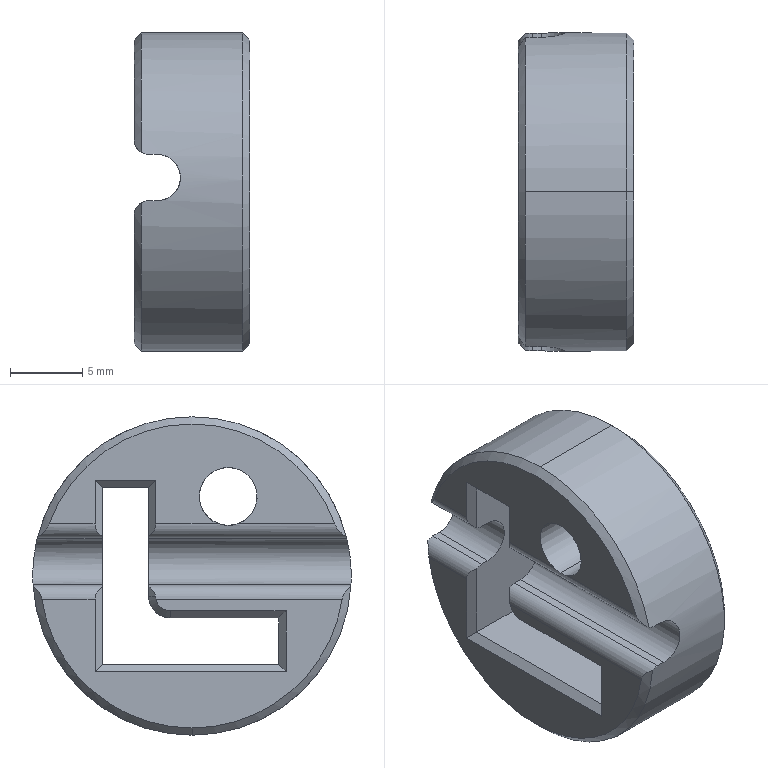Part | SolidWorks | features BaseBody 1 | 1 solid | 45 faces | box 8 x 22 x 22 mm | volume 2188 mm3 | plane 27 | cylinder 11 | cone 7 | commonest cylinder face diameters 2 x4 3.2 x2 4 x2 22 x2 3 x1
STEP:
#1=CARTESIAN_POINT('',(16.,98.,-26.5));
#2=VERTEX_POINT('',#1);
#3=CARTESIAN_POINT('',(16.,98.,-5.5));
#4=VERTEX_POINT('',#3);
#5=CARTESIAN_POINT('',(16.,98.,-16.));
#6=DIRECTION('',(1.,0.,0.));
#7=DIRECTION('',(0.,0.,1.));
#8=AXIS2_PLACEMENT_3D('',#5,#6,#7);
#9=CIRCLE('',#8,10.5);
#10=EDGE_CURVE('',#2,#4,#9,.T.);
#11=ORIENTED_EDGE('',*,*,#10,.F.);
#12=CARTESIAN_POINT('',(15.5,98.,-27.));
#13=VERTEX_POINT('',#12);
#14=CARTESIAN_POINT('',(15.5,98.,-27.));
#15=DIRECTION('',(-0.7071,0.,-0.7071));
#16=VECTOR('',#15,1000.);
#17=LINE('',#14,#16);
#18=EDGE_CURVE('',#2,#13,#17,.T.);
#19=ORIENTED_EDGE('',*,*,#18,.T.);
#20=CARTESIAN_POINT('',(15.5,98.,-5.));
#21=VERTEX_POINT('',#20);
#22=CARTESIAN_POINT('',(15.5,98.,-16.));
#23=DIRECTION('',(-1.,0.,0.));
#24=DIRECTION('',(0.,0.,1.));
#25=AXIS2_PLACEMENT_3D('',#22,#23,#24);
#26=CIRCLE('',#25,11.);
#27=EDGE_CURVE('',#21,#13,#26,.T.);
#28=ORIENTED_EDGE('',*,*,#27,.F.);
#29=CARTESIAN_POINT('',(15.5,98.,-5.));
#30=DIRECTION('',(-0.7071,0.,0.7071));
#31=VECTOR('',#30,1000.);
#32=LINE('',#29,#31);
#33=EDGE_CURVE('',#4,#21,#32,.T.);
#34=ORIENTED_EDGE('',*,*,#33,.F.);
#35=EDGE_LOOP('',(#11,#19,#28,#34));
#36=FACE_OUTER_BOUND('',#35,.T.);
#37=CARTESIAN_POINT('',(15.5,98.,-16.));
#38=DIRECTION('',(-1.,0.,0.));
#39=DIRECTION('',(0.,0.,1.));
#40=AXIS2_PLACEMENT_3D('',#37,#38,#39);
#41=CONICAL_SURFACE('',#40,11.,0.7854);
#42=ADVANCED_FACE('',(#36),#41,.T.);
#43=CARTESIAN_POINT('',(8.,94.876,-12.4));
#44=VERTEX_POINT('',#43);
#45=CARTESIAN_POINT('',(8.,95.5,-8.5));
#46=VERTEX_POINT('',#45);
#47=CARTESIAN_POINT('',(8.,95.5,-10.5));
#48=DIRECTION('',(-1.,0.,0.));
#49=DIRECTION('',(0.,0.,1.));
#50=AXIS2_PLACEMENT_3D('',#47,#48,#49);
#51=CIRCLE('',#50,2.);
#52=EDGE_CURVE('',#44,#46,#51,.T.);
#53=ORIENTED_EDGE('',*,*,#52,.T.);
#54=CARTESIAN_POINT('',(16.,95.5,-8.5));
#55=VERTEX_POINT('',#54);
#56=CARTESIAN_POINT('',(8.,95.5,-8.5));
#57=DIRECTION('',(1.,0.,0.));
#58=VECTOR('',#57,1000.);
#59=LINE('',#56,#58);
#60=EDGE_CURVE('',#46,#55,#59,.T.);
#61=ORIENTED_EDGE('',*,*,#60,.T.);
#62=CARTESIAN_POINT('',(16.,95.5,-12.5));
#63=VERTEX_POINT('',#62);
#64=CARTESIAN_POINT('',(16.,95.5,-10.5));
#65=DIRECTION('',(-1.,0.,0.));
#66=DIRECTION('',(0.,0.,1.));
#67=AXIS2_PLACEMENT_3D('',#64,#65,#66);
#68=CIRCLE('',#67,2.);
#69=EDGE_CURVE('',#63,#55,#68,.T.);
#70=ORIENTED_EDGE('',*,*,#69,.F.);
#71=CARTESIAN_POINT('',(8.005,95.5,-12.5));
#72=VERTEX_POINT('',#71);
#73=CARTESIAN_POINT('',(8.,95.5,-12.5));
#74=DIRECTION('',(1.,0.,0.));
#75=VECTOR('',#74,1000.);
#76=LINE('',#73,#75);
#77=EDGE_CURVE('',#72,#63,#76,.T.);
#78=ORIENTED_EDGE('',*,*,#77,.F.);
#79=CARTESIAN_POINT('',(8.005,95.5,-12.5));
#80=CARTESIAN_POINT('',(8.005,95.287,-12.5));
#81=CARTESIAN_POINT('',(8.,95.078,-12.467));
#82=CARTESIAN_POINT('',(8.,94.876,-12.4));
#83=B_SPLINE_CURVE_WITH_KNOTS('',3,(#79,#80,#81,#82),.UNSPECIFIED.,.F.,.F.,(4,4),(0.0006324,0.001263),.UNSPECIFIED.);
#84=EDGE_CURVE('',#72,#44,#83,.T.);
#85=ORIENTED_EDGE('',*,*,#84,.T.);
#86=EDGE_LOOP('',(#53,#61,#70,#78,#85));
#87=FACE_OUTER_BOUND('',#86,.T.);
#88=CARTESIAN_POINT('',(8.,95.5,-10.5));
#89=DIRECTION('',(1.,0.,0.));
#90=DIRECTION('',(0.,0.,-1.));
#91=AXIS2_PLACEMENT_3D('',#88,#89,#90);
#92=CYLINDRICAL_SURFACE('',#91,2.);
#93=ADVANCED_FACE('',(#87),#92,.F.);
#94=CARTESIAN_POINT('',(8.5,108.655,-13.266));
#95=VERTEX_POINT('',#94);
#96=CARTESIAN_POINT('',(8.5,98.,-5.));
#97=VERTEX_POINT('',#96);
#98=CARTESIAN_POINT('',(8.5,98.,-16.));
#99=DIRECTION('',(1.,0.,0.));
#100=DIRECTION('',(0.,0.,1.));
#101=AXIS2_PLACEMENT_3D('',#98,#99,#100);
#102=CIRCLE('',#101,11.);
#103=EDGE_CURVE('',#95,#97,#102,.T.);
#104=ORIENTED_EDGE('',*,*,#103,.T.);
#105=CARTESIAN_POINT('',(8.,98.,-5.));
#106=DIRECTION('',(1.,0.,0.));
#107=VECTOR('',#106,1000.);
#108=LINE('',#105,#107);
#109=EDGE_CURVE('',#97,#21,#108,.T.);
#110=ORIENTED_EDGE('',*,*,#109,.T.);
#111=ORIENTED_EDGE('',*,*,#27,.T.);
#112=CARTESIAN_POINT('',(8.5,98.,-27.));
#113=VERTEX_POINT('',#112);
#114=CARTESIAN_POINT('',(8.,98.,-27.));
#115=DIRECTION('',(1.,0.,0.));
#116=VECTOR('',#115,1000.);
#117=LINE('',#114,#116);
#118=EDGE_CURVE('',#113,#13,#117,.T.);
#119=ORIENTED_EDGE('',*,*,#118,.F.);
#120=CARTESIAN_POINT('',(8.5,108.975,-16.734));
#121=VERTEX_POINT('',#120);
#122=CARTESIAN_POINT('',(8.5,98.,-16.));
#123=DIRECTION('',(1.,0.,0.));
#124=DIRECTION('',(0.,0.,1.));
#125=AXIS2_PLACEMENT_3D('',#122,#123,#124);
#126=CIRCLE('',#125,11.);
#127=EDGE_CURVE('',#113,#121,#126,.T.);
#128=ORIENTED_EDGE('',*,*,#127,.T.);
#129=CARTESIAN_POINT('',(9.,108.984,-16.6));
#130=VERTEX_POINT('',#129);
#131=CARTESIAN_POINT('',(8.5,108.975,-16.734));
#132=CARTESIAN_POINT('',(8.652,108.981,-16.646));
#133=CARTESIAN_POINT('',(8.824,108.984,-16.6));
#134=CARTESIAN_POINT('',(9.,108.984,-16.6));
#135=B_SPLINE_CURVE_WITH_KNOTS('',3,(#131,#132,#133,#134),.UNSPECIFIED.,.F.,.F.,(4,4),(0.,0.00052),.UNSPECIFIED.);
#136=EDGE_CURVE('',#121,#130,#135,.T.);
#137=ORIENTED_EDGE('',*,*,#136,.T.);
#138=CARTESIAN_POINT('',(9.6,108.984,-16.6));
#139=VERTEX_POINT('',#138);
#140=CARTESIAN_POINT('',(8.,108.984,-16.6));
#141=DIRECTION('',(1.,0.,0.));
#142=VECTOR('',#141,1000.);
#143=LINE('',#140,#142);
#144=EDGE_CURVE('',#130,#139,#143,.T.);
#145=ORIENTED_EDGE('',*,*,#144,.T.);
#146=CARTESIAN_POINT('',(9.6,108.688,-13.4));
#147=VERTEX_POINT('',#146);
#148=CARTESIAN_POINT('',(9.6,108.984,-16.6));
#149=CARTESIAN_POINT('',(9.706,108.984,-16.6));
#150=CARTESIAN_POINT('',(9.81,108.984,-16.59));
#151=CARTESIAN_POINT('',(10.015,108.986,-16.549));
#152=CARTESIAN_POINT('',(10.117,108.988,-16.518));
#153=CARTESIAN_POINT('',(10.312,108.991,-16.437));
#154=CARTESIAN_POINT('',(10.404,108.993,-16.387));
#155=CARTESIAN_POINT('',(10.578,108.997,-16.271));
#156=CARTESIAN_POINT('',(10.661,108.998,-16.203));
#157=CARTESIAN_POINT('',(10.882,109.001,-15.98));
#158=CARTESIAN_POINT('',(11.001,109.,-15.8));
#159=CARTESIAN_POINT('',(11.16,108.986,-15.414));
#160=CARTESIAN_POINT('',(11.201,108.973,-15.202));
#161=CARTESIAN_POINT('',(11.2,108.944,-14.889));
#162=CARTESIAN_POINT('',(11.189,108.933,-14.784));
#163=CARTESIAN_POINT('',(11.147,108.908,-14.58));
#164=CARTESIAN_POINT('',(11.117,108.895,-14.48));
#165=CARTESIAN_POINT('',(10.996,108.852,-14.191));
#166=CARTESIAN_POINT('',(10.88,108.821,-14.017));
#167=CARTESIAN_POINT('',(10.657,108.777,-13.794));
#168=CARTESIAN_POINT('',(10.577,108.763,-13.728));
#169=CARTESIAN_POINT('',(10.404,108.738,-13.613));
#170=CARTESIAN_POINT('',(10.311,108.727,-13.563));
#171=CARTESIAN_POINT('',(10.021,108.699,-13.442));
#172=CARTESIAN_POINT('',(9.812,108.688,-13.4));
#173=CARTESIAN_POINT('',(9.6,108.688,-13.4));
#174=B_SPLINE_CURVE_WITH_KNOTS('',3,(#148,#149,#150,#151,#152,#153,#154,#155,#156,#157,#158,#159,#160,#161,#162,#163,#164,#165,#166,#167,#168,#169,#170,#171,#172,#173),.UNSPECIFIED.,.F.,.F.,(4,2,2,2,2,2,2,2,2,2,2,2,4),(0.,0.0003137,0.0006273,0.000941,0.001255,0.001882,0.002509,0.002823,0.003137,0.003764,0.004078,0.004391,0.005019),.UNSPECIFIED.);
#175=EDGE_CURVE('',#139,#147,#174,.T.);
#176=ORIENTED_EDGE('',*,*,#175,.T.);
#177=CARTESIAN_POINT('',(9.,108.688,-13.4));
#178=VERTEX_POINT('',#177);
#179=CARTESIAN_POINT('',(8.,108.688,-13.4));
#180=DIRECTION('',(-1.,0.,0.));
#181=VECTOR('',#180,1000.);
#182=LINE('',#179,#181);
#183=EDGE_CURVE('',#147,#178,#182,.T.);
#184=ORIENTED_EDGE('',*,*,#183,.T.);
#185=CARTESIAN_POINT('',(9.,108.688,-13.4));
#186=CARTESIAN_POINT('',(8.824,108.688,-13.4));
#187=CARTESIAN_POINT('',(8.651,108.677,-13.353));
#188=CARTESIAN_POINT('',(8.5,108.655,-13.266));
#189=B_SPLINE_CURVE_WITH_KNOTS('',3,(#185,#186,#187,#188),.UNSPECIFIED.,.F.,.F.,(4,4),(0.,0.0005213),.UNSPECIFIED.);
#190=EDGE_CURVE('',#178,#95,#189,.T.);
#191=ORIENTED_EDGE('',*,*,#190,.T.);
#192=EDGE_LOOP('',(#104,#110,#111,#119,#128,#137,#145,#176,#184,#191));
#193=FACE_OUTER_BOUND('',#192,.T.);
#194=CARTESIAN_POINT('',(8.,98.,-16.));
#195=DIRECTION('',(1.,0.,0.));
#196=DIRECTION('',(0.,0.,-1.));
#197=AXIS2_PLACEMENT_3D('',#194,#195,#196);
#198=CYLINDRICAL_SURFACE('',#197,11.);
#199=ADVANCED_FACE('',(#193),#198,.T.);
#200=CARTESIAN_POINT('',(8.,98.,-26.5));
#201=VERTEX_POINT('',#200);
#202=CARTESIAN_POINT('',(8.,87.623,-17.6));
#203=VERTEX_POINT('',#202);
#204=CARTESIAN_POINT('',(8.,98.,-16.));
#205=DIRECTION('',(-1.,0.,0.));
#206=DIRECTION('',(0.,0.,1.));
#207=AXIS2_PLACEMENT_3D('',#204,#205,#206);
#208=CIRCLE('',#207,10.5);
#209=EDGE_CURVE('',#201,#203,#208,.T.);
#210=ORIENTED_EDGE('',*,*,#209,.F.);
#211=CARTESIAN_POINT('',(8.,98.,-26.5));
#212=DIRECTION('',(0.7071,0.,-0.7071));
#213=VECTOR('',#212,1000.);
#214=LINE('',#211,#213);
#215=EDGE_CURVE('',#201,#113,#214,.T.);
#216=ORIENTED_EDGE('',*,*,#215,.T.);
#217=CARTESIAN_POINT('',(8.5,87.025,-16.734));
#218=VERTEX_POINT('',#217);
#219=CARTESIAN_POINT('',(8.5,98.,-16.));
#220=DIRECTION('',(1.,0.,0.));
#221=DIRECTION('',(0.,0.,1.));
#222=AXIS2_PLACEMENT_3D('',#219,#220,#221);
#223=CIRCLE('',#222,11.);
#224=EDGE_CURVE('',#218,#113,#223,.T.);
#225=ORIENTED_EDGE('',*,*,#224,.F.);
#226=CARTESIAN_POINT('',(8.5,87.025,-16.734));
#227=CARTESIAN_POINT('',(8.434,87.093,-16.772));
#228=CARTESIAN_POINT('',(8.372,87.159,-16.818));
#229=CARTESIAN_POINT('',(8.256,87.284,-16.927));
#230=CARTESIAN_POINT('',(8.202,87.344,-16.991));
#231=CARTESIAN_POINT('',(8.063,87.505,-17.21));
#232=CARTESIAN_POINT('',(8.,87.591,-17.396));
#233=CARTESIAN_POINT('',(8.,87.623,-17.6));
#234=B_SPLINE_CURVE_WITH_KNOTS('',3,(#226,#227,#228,#229,#230,#231,#232,#233),.UNSPECIFIED.,.F.,.F.,(4,2,2,4),(0.,0.0003033,0.0006065,0.001213),.UNSPECIFIED.);
#235=EDGE_CURVE('',#218,#203,#234,.T.);
#236=ORIENTED_EDGE('',*,*,#235,.T.);
#237=EDGE_LOOP('',(#210,#216,#225,#236));
#238=FACE_OUTER_BOUND('',#237,.T.);
#239=CARTESIAN_POINT('',(8.,98.,-16.));
#240=DIRECTION('',(1.,0.,0.));
#241=DIRECTION('',(0.,0.,-1.));
#242=AXIS2_PLACEMENT_3D('',#239,#240,#241);
#243=CONICAL_SURFACE('',#242,10.5,0.7854);
#244=ADVANCED_FACE('',(#238),#243,.T.);
#245=CARTESIAN_POINT('',(8.,108.377,-17.6));
#246=VERTEX_POINT('',#245);
#247=CARTESIAN_POINT('',(8.,98.,-16.));
#248=DIRECTION('',(-1.,0.,0.));
#249=DIRECTION('',(0.,0.,1.));
#250=AXIS2_PLACEMENT_3D('',#247,#248,#249);
#251=CIRCLE('',#250,10.5);
#252=EDGE_CURVE('',#246,#201,#251,.T.);
#253=ORIENTED_EDGE('',*,*,#252,.T.);
#254=ORIENTED_EDGE('',*,*,#209,.T.);
#255=CARTESIAN_POINT('',(8.,100.48,-17.6));
#256=VERTEX_POINT('',#255);
#257=CARTESIAN_POINT('',(8.,100.5,-17.6));
#258=DIRECTION('',(0.,1.,0.));
#259=VECTOR('',#258,1000.);
#260=LINE('',#257,#259);
#261=EDGE_CURVE('',#203,#256,#260,.T.);
#262=ORIENTED_EDGE('',*,*,#261,.T.);
#263=CARTESIAN_POINT('',(8.,99.5,-18.4));
#264=VERTEX_POINT('',#263);
#265=CARTESIAN_POINT('',(8.,99.5,-17.4));
#266=DIRECTION('',(-1.,0.,0.));
#267=DIRECTION('',(0.,0.,1.));
#268=AXIS2_PLACEMENT_3D('',#265,#266,#267);
#269=CIRCLE('',#268,1.);
#270=EDGE_CURVE('',#256,#264,#269,.T.);
#271=ORIENTED_EDGE('',*,*,#270,.T.);
#272=CARTESIAN_POINT('',(8.,91.5,-18.4));
#273=VERTEX_POINT('',#272);
#274=CARTESIAN_POINT('',(8.,98.,-18.4));
#275=DIRECTION('',(0.,-1.,0.));
#276=VECTOR('',#275,1000.);
#277=LINE('',#274,#276);
#278=EDGE_CURVE('',#264,#273,#277,.T.);
#279=ORIENTED_EDGE('',*,*,#278,.T.);
#280=CARTESIAN_POINT('',(8.,91.5,-22.6));
#281=VERTEX_POINT('',#280);
#282=CARTESIAN_POINT('',(8.,91.5,-16.));
#283=DIRECTION('',(0.,0.,-1.));
#284=VECTOR('',#283,1000.);
#285=LINE('',#282,#284);
#286=EDGE_CURVE('',#273,#281,#285,.T.);
#287=ORIENTED_EDGE('',*,*,#286,.T.);
#288=CARTESIAN_POINT('',(8.,104.7,-22.6));
#289=VERTEX_POINT('',#288);
#290=CARTESIAN_POINT('',(8.,98.,-22.6));
#291=DIRECTION('',(0.,1.,0.));
#292=VECTOR('',#291,1000.);
#293=LINE('',#290,#292);
#294=EDGE_CURVE('',#281,#289,#293,.T.);
#295=ORIENTED_EDGE('',*,*,#294,.T.);
#296=CARTESIAN_POINT('',(8.,104.7,-17.6));
#297=VERTEX_POINT('',#296);
#298=CARTESIAN_POINT('',(8.,104.7,-16.));
#299=DIRECTION('',(0.,0.,1.));
#300=VECTOR('',#299,1000.);
#301=LINE('',#298,#300);
#302=EDGE_CURVE('',#289,#297,#301,.T.);
#303=ORIENTED_EDGE('',*,*,#302,.T.);
#304=CARTESIAN_POINT('',(8.,108.483,-17.6));
#305=DIRECTION('',(0.,1.,0.));
#306=VECTOR('',#305,1000.);
#307=LINE('',#304,#306);
#308=EDGE_CURVE('',#297,#246,#307,.T.);
#309=ORIENTED_EDGE('',*,*,#308,.T.);
#310=EDGE_LOOP('',(#253,#254,#262,#271,#279,#287,#295,#303,#309));
#311=FACE_OUTER_BOUND('',#310,.T.);
#312=CARTESIAN_POINT('',(8.,98.,-16.));
#313=DIRECTION('',(-1.,0.,0.));
#314=DIRECTION('',(0.,0.,1.));
#315=AXIS2_PLACEMENT_3D('',#312,#313,#314);
#316=PLANE('',#315);
#317=ADVANCED_FACE('',(#311),#316,.T.);
#318=ORIENTED_EDGE('',*,*,#215,.F.);
#319=ORIENTED_EDGE('',*,*,#252,.F.);
#320=CARTESIAN_POINT('',(8.,108.377,-17.6));
#321=CARTESIAN_POINT('',(8.,108.409,-17.396));
#322=CARTESIAN_POINT('',(8.062,108.493,-17.212));
#323=CARTESIAN_POINT('',(8.248,108.71,-16.918));
#324=CARTESIAN_POINT('',(8.368,108.838,-16.81));
#325=CARTESIAN_POINT('',(8.5,108.975,-16.734));
#326=B_SPLINE_CURVE_WITH_KNOTS('',3,(#320,#321,#322,#323,#324,#325),.UNSPECIFIED.,.F.,.F.,(4,2,4),(0.,0.0006077,0.001215),.UNSPECIFIED.);
#327=EDGE_CURVE('',#246,#121,#326,.T.);
#328=ORIENTED_EDGE('',*,*,#327,.T.);
#329=ORIENTED_EDGE('',*,*,#127,.F.);
#330=EDGE_LOOP('',(#318,#319,#328,#329));
#331=FACE_OUTER_BOUND('',#330,.T.);
#332=CARTESIAN_POINT('',(8.,98.,-16.));
#333=DIRECTION('',(1.,0.,0.));
#334=DIRECTION('',(0.,0.,-1.));
#335=AXIS2_PLACEMENT_3D('',#332,#333,#334);
#336=CONICAL_SURFACE('',#335,10.5,0.7854);
#337=ADVANCED_FACE('',(#331),#336,.T.);
#338=CARTESIAN_POINT('',(8.02,100.52,-17.4));
#339=VERTEX_POINT('',#338);
#340=CARTESIAN_POINT('',(8.5,101.,-17.4));
#341=VERTEX_POINT('',#340);
#342=CARTESIAN_POINT('',(8.,100.5,-17.4));
#343=DIRECTION('',(0.7071,0.7071,0.));
#344=VECTOR('',#343,1000.);
#345=LINE('',#342,#344);
#346=EDGE_CURVE('',#339,#341,#345,.T.);
#347=ORIENTED_EDGE('',*,*,#346,.F.);
#348=CARTESIAN_POINT('',(8.5,101.,-16.734));
#349=VERTEX_POINT('',#348);
#350=CARTESIAN_POINT('',(8.02,100.52,-17.4));
#351=CARTESIAN_POINT('',(8.078,100.578,-17.115));
#352=CARTESIAN_POINT('',(8.248,100.748,-16.879));
#353=CARTESIAN_POINT('',(8.5,101.,-16.734));
#354=(BOUNDED_CURVE()B_SPLINE_CURVE(3,(#350,#351,#352,#353),.UNSPECIFIED.,.F.,.F.)B_SPLINE_CURVE_WITH_KNOTS((4,4),(0.2014,1.047),.UNSPECIFIED.)CURVE()GEOMETRIC_REPRESENTATION_ITEM()RATIONAL_B_SPLINE_CURVE((1.,0.9413,0.9413,1.))REPRESENTATION_ITEM(''));
#355=EDGE_CURVE('',#339,#349,#354,.T.);
#356=ORIENTED_EDGE('',*,*,#355,.T.);
#357=CARTESIAN_POINT('',(8.5,101.,-17.4));
#358=DIRECTION('',(0.,0.,1.));
#359=VECTOR('',#358,1000.);
#360=LINE('',#357,#359);
#361=EDGE_CURVE('',#341,#349,#360,.T.);
#362=ORIENTED_EDGE('',*,*,#361,.F.);
#363=EDGE_LOOP('',(#347,#356,#362));
#364=FACE_OUTER_BOUND('',#363,.T.);
#365=CARTESIAN_POINT('',(8.5,101.,-17.4));
#366=DIRECTION('',(0.7071,-0.7071,0.));
#367=DIRECTION('',(0.7071,0.7071,0.));
#368=AXIS2_PLACEMENT_3D('',#365,#366,#367);
#369=PLANE('',#368);
#370=ADVANCED_FACE('',(#364),#369,.F.);
#371=CARTESIAN_POINT('',(8.5,104.2,-16.734));
#372=VERTEX_POINT('',#371);
#373=CARTESIAN_POINT('',(8.5,104.2,-22.1));
#374=VERTEX_POINT('',#373);
#375=CARTESIAN_POINT('',(8.5,104.2,-22.1));
#376=DIRECTION('',(0.,0.,-1.));
#377=VECTOR('',#376,1000.);
#378=LINE('',#375,#377);
#379=EDGE_CURVE('',#372,#374,#378,.T.);
#380=ORIENTED_EDGE('',*,*,#379,.F.);
#381=CARTESIAN_POINT('',(8.5,104.2,-16.734));
#382=CARTESIAN_POINT('',(8.183,104.517,-16.917));
#383=CARTESIAN_POINT('',(8.,104.7,-17.234));
#384=CARTESIAN_POINT('',(8.,104.7,-17.6));
#385=(BOUNDED_CURVE()B_SPLINE_CURVE(3,(#381,#382,#383,#384),.UNSPECIFIED.,.F.,.F.)B_SPLINE_CURVE_WITH_KNOTS((4,4),(2.094,3.142),.UNSPECIFIED.)CURVE()GEOMETRIC_REPRESENTATION_ITEM()RATIONAL_B_SPLINE_CURVE((1.,0.9107,0.9107,1.))REPRESENTATION_ITEM(''));
#386=EDGE_CURVE('',#372,#297,#385,.T.);
#387=ORIENTED_EDGE('',*,*,#386,.T.);
#388=ORIENTED_EDGE('',*,*,#302,.F.);
#389=CARTESIAN_POINT('',(8.5,104.2,-22.1));
#390=DIRECTION('',(-0.5774,0.5774,-0.5774));
#391=VECTOR('',#390,1000.);
#392=LINE('',#389,#391);
#393=EDGE_CURVE('',#374,#289,#392,.T.);
#394=ORIENTED_EDGE('',*,*,#393,.F.);
#395=EDGE_LOOP('',(#380,#387,#388,#394));
#396=FACE_OUTER_BOUND('',#395,.T.);
#397=CARTESIAN_POINT('',(8.5,104.2,-22.1));
#398=DIRECTION('',(0.7071,0.7071,0.));
#399=DIRECTION('',(-0.7071,0.7071,0.));
#400=AXIS2_PLACEMENT_3D('',#397,#398,#399);
#401=PLANE('',#400);
#402=ADVANCED_FACE('',(#396),#401,.F.);
#403=CARTESIAN_POINT('',(8.,88.136,-12.4));
#404=VERTEX_POINT('',#403);
#405=CARTESIAN_POINT('',(8.,107.864,-12.4));
#406=VERTEX_POINT('',#405);
#407=CARTESIAN_POINT('',(8.,98.,-16.));
#408=DIRECTION('',(-1.,0.,0.));
#409=DIRECTION('',(0.,0.,1.));
#410=AXIS2_PLACEMENT_3D('',#407,#408,#409);
#411=CIRCLE('',#410,10.5);
#412=EDGE_CURVE('',#404,#406,#411,.T.);
#413=ORIENTED_EDGE('',*,*,#412,.T.);
#414=CARTESIAN_POINT('',(8.,104.7,-12.4));
#415=VERTEX_POINT('',#414);
#416=CARTESIAN_POINT('',(8.,104.7,-12.4));
#417=DIRECTION('',(0.,-1.,0.));
#418=VECTOR('',#417,1000.);
#419=LINE('',#416,#418);
#420=EDGE_CURVE('',#406,#415,#419,.T.);
#421=ORIENTED_EDGE('',*,*,#420,.T.);
#422=CARTESIAN_POINT('',(8.,104.7,-9.4));
#423=VERTEX_POINT('',#422);
#424=CARTESIAN_POINT('',(8.,104.7,-16.));
#425=DIRECTION('',(0.,0.,1.));
#426=VECTOR('',#425,1000.);
#427=LINE('',#424,#426);
#428=EDGE_CURVE('',#415,#423,#427,.T.);
#429=ORIENTED_EDGE('',*,*,#428,.T.);
#430=CARTESIAN_POINT('',(8.,100.5,-9.4));
#431=VERTEX_POINT('',#430);
#432=CARTESIAN_POINT('',(8.,98.,-9.4));
#433=DIRECTION('',(0.,-1.,0.));
#434=VECTOR('',#433,1000.);
#435=LINE('',#432,#434);
#436=EDGE_CURVE('',#423,#431,#435,.T.);
#437=ORIENTED_EDGE('',*,*,#436,.T.);
#438=CARTESIAN_POINT('',(8.,100.5,-12.4));
#439=VERTEX_POINT('',#438);
#440=CARTESIAN_POINT('',(8.,100.5,-16.));
#441=DIRECTION('',(0.,0.,-1.));
#442=VECTOR('',#441,1000.);
#443=LINE('',#440,#442);
#444=EDGE_CURVE('',#431,#439,#443,.T.);
#445=ORIENTED_EDGE('',*,*,#444,.T.);
#446=CARTESIAN_POINT('',(8.,96.124,-12.4));
#447=VERTEX_POINT('',#446);
#448=CARTESIAN_POINT('',(8.,87.827,-12.4));
#449=DIRECTION('',(0.,-1.,0.));
#450=VECTOR('',#449,1000.);
#451=LINE('',#448,#450);
#452=EDGE_CURVE('',#439,#447,#451,.T.);
#453=ORIENTED_EDGE('',*,*,#452,.T.);
#454=CARTESIAN_POINT('',(8.,95.5,-10.5));
#455=DIRECTION('',(-1.,0.,0.));
#456=DIRECTION('',(0.,0.,1.));
#457=AXIS2_PLACEMENT_3D('',#454,#455,#456);
#458=CIRCLE('',#457,2.);
#459=EDGE_CURVE('',#46,#447,#458,.T.);
#460=ORIENTED_EDGE('',*,*,#459,.F.);
#461=ORIENTED_EDGE('',*,*,#52,.F.);
#462=CARTESIAN_POINT('',(8.,87.827,-12.4));
#463=DIRECTION('',(0.,-1.,0.));
#464=VECTOR('',#463,1000.);
#465=LINE('',#462,#464);
#466=EDGE_CURVE('',#44,#404,#465,.T.);
#467=ORIENTED_EDGE('',*,*,#466,.T.);
#468=EDGE_LOOP('',(#413,#421,#429,#437,#445,#453,#460,#461,#467));
#469=FACE_OUTER_BOUND('',#468,.T.);
#470=CARTESIAN_POINT('',(8.,98.,-16.));
#471=DIRECTION('',(-1.,0.,0.));
#472=DIRECTION('',(0.,0.,1.));
#473=AXIS2_PLACEMENT_3D('',#470,#471,#472);
#474=PLANE('',#473);
#475=ADVANCED_FACE('',(#469),#474,.T.);
#476=CARTESIAN_POINT('',(16.,98.,-16.));
#477=DIRECTION('',(1.,0.,0.));
#478=DIRECTION('',(0.,0.,1.));
#479=AXIS2_PLACEMENT_3D('',#476,#477,#478);
#480=CIRCLE('',#479,10.5);
#481=EDGE_CURVE('',#4,#2,#480,.T.);
#482=ORIENTED_EDGE('',*,*,#481,.T.);
#483=ORIENTED_EDGE('',*,*,#10,.T.);
#484=EDGE_LOOP('',(#482,#483));
#485=FACE_OUTER_BOUND('',#484,.T.);
#486=CARTESIAN_POINT('',(16.,100.5,-9.4));
#487=VERTEX_POINT('',#486);
#488=CARTESIAN_POINT('',(16.,104.7,-9.4));
#489=VERTEX_POINT('',#488);
#490=CARTESIAN_POINT('',(16.,104.2,-9.4));
#491=DIRECTION('',(0.,1.,0.));
#492=VECTOR('',#491,1000.);
#493=LINE('',#490,#492);
#494=EDGE_CURVE('',#487,#489,#493,.T.);
#495=ORIENTED_EDGE('',*,*,#494,.T.);
#496=CARTESIAN_POINT('',(16.,104.7,-22.6));
#497=VERTEX_POINT('',#496);
#498=CARTESIAN_POINT('',(16.,104.7,-22.1));
#499=DIRECTION('',(0.,0.,-1.));
#500=VECTOR('',#499,1000.);
#501=LINE('',#498,#500);
#502=EDGE_CURVE('',#489,#497,#501,.T.);
#503=ORIENTED_EDGE('',*,*,#502,.T.);
#504=CARTESIAN_POINT('',(16.,91.5,-22.6));
#505=VERTEX_POINT('',#504);
#506=CARTESIAN_POINT('',(16.,92.,-22.6));
#507=DIRECTION('',(0.,-1.,0.));
#508=VECTOR('',#507,1000.);
#509=LINE('',#506,#508);
#510=EDGE_CURVE('',#497,#505,#509,.T.);
#511=ORIENTED_EDGE('',*,*,#510,.T.);
#512=CARTESIAN_POINT('',(16.,91.5,-18.4));
#513=VERTEX_POINT('',#512);
#514=CARTESIAN_POINT('',(16.,91.5,-18.9));
#515=DIRECTION('',(0.,0.,1.));
#516=VECTOR('',#515,1000.);
#517=LINE('',#514,#516);
#518=EDGE_CURVE('',#505,#513,#517,.T.);
#519=ORIENTED_EDGE('',*,*,#518,.T.);
#520=CARTESIAN_POINT('',(16.,99.5,-18.4));
#521=VERTEX_POINT('',#520);
#522=CARTESIAN_POINT('',(16.,99.5,-18.4));
#523=DIRECTION('',(0.,1.,0.));
#524=VECTOR('',#523,1000.);
#525=LINE('',#522,#524);
#526=EDGE_CURVE('',#513,#521,#525,.T.);
#527=ORIENTED_EDGE('',*,*,#526,.T.);
#528=CARTESIAN_POINT('',(16.,100.5,-17.4));
#529=VERTEX_POINT('',#528);
#530=CARTESIAN_POINT('',(16.,99.5,-17.4));
#531=DIRECTION('',(1.,0.,0.));
#532=DIRECTION('',(0.,0.,1.));
#533=AXIS2_PLACEMENT_3D('',#530,#531,#532);
#534=CIRCLE('',#533,1.);
#535=EDGE_CURVE('',#521,#529,#534,.T.);
#536=ORIENTED_EDGE('',*,*,#535,.T.);
#537=CARTESIAN_POINT('',(16.,100.5,-9.9));
#538=DIRECTION('',(0.,0.,1.));
#539=VECTOR('',#538,1000.);
#540=LINE('',#537,#539);
#541=EDGE_CURVE('',#529,#487,#540,.T.);
#542=ORIENTED_EDGE('',*,*,#541,.T.);
#543=EDGE_LOOP('',(#495,#503,#511,#519,#527,#536,#542));
#544=FACE_BOUND('',#543,.T.);
#545=ORIENTED_EDGE('',*,*,#69,.T.);
#546=CARTESIAN_POINT('',(16.,95.5,-10.5));
#547=DIRECTION('',(-1.,0.,0.));
#548=DIRECTION('',(0.,0.,1.));
#549=AXIS2_PLACEMENT_3D('',#546,#547,#548);
#550=CIRCLE('',#549,2.);
#551=EDGE_CURVE('',#55,#63,#550,.T.);
#552=ORIENTED_EDGE('',*,*,#551,.T.);
#553=EDGE_LOOP('',(#545,#552));
#554=FACE_BOUND('',#553,.T.);
#555=CARTESIAN_POINT('',(16.,98.,-16.));
#556=DIRECTION('',(-1.,0.,0.));
#557=DIRECTION('',(0.,0.,1.));
#558=AXIS2_PLACEMENT_3D('',#555,#556,#557);
#559=PLANE('',#558);
#560=ADVANCED_FACE('',(#485,#544,#554),#559,.F.);
#561=ORIENTED_EDGE('',*,*,#109,.F.);
#562=CARTESIAN_POINT('',(8.5,87.345,-13.266));
#563=VERTEX_POINT('',#562);
#564=CARTESIAN_POINT('',(8.5,98.,-16.));
#565=DIRECTION('',(1.,0.,0.));
#566=DIRECTION('',(0.,0.,1.));
#567=AXIS2_PLACEMENT_3D('',#564,#565,#566);
#568=CIRCLE('',#567,11.);
#569=EDGE_CURVE('',#97,#563,#568,.T.);
#570=ORIENTED_EDGE('',*,*,#569,.T.);
#571=CARTESIAN_POINT('',(9.,87.312,-13.4));
#572=VERTEX_POINT('',#571);
#573=CARTESIAN_POINT('',(8.5,87.345,-13.266));
#574=CARTESIAN_POINT('',(8.651,87.323,-13.353));
#575=CARTESIAN_POINT('',(8.824,87.312,-13.4));
#576=CARTESIAN_POINT('',(9.,87.312,-13.4));
#577=B_SPLINE_CURVE_WITH_KNOTS('',3,(#573,#574,#575,#576),.UNSPECIFIED.,.F.,.F.,(4,4),(0.,0.0005213),.UNSPECIFIED.);
#578=EDGE_CURVE('',#563,#572,#577,.T.);
#579=ORIENTED_EDGE('',*,*,#578,.T.);
#580=CARTESIAN_POINT('',(9.6,87.312,-13.4));
#581=VERTEX_POINT('',#580);
#582=CARTESIAN_POINT('',(8.,87.312,-13.4));
#583=DIRECTION('',(1.,0.,0.));
#584=VECTOR('',#583,1000.);
#585=LINE('',#582,#584);
#586=EDGE_CURVE('',#572,#581,#585,.T.);
#587=ORIENTED_EDGE('',*,*,#586,.T.);
#588=CARTESIAN_POINT('',(9.6,87.016,-16.6));
#589=VERTEX_POINT('',#588);
#590=CARTESIAN_POINT('',(9.6,87.312,-13.4));
#591=CARTESIAN_POINT('',(9.706,87.312,-13.4));
#592=CARTESIAN_POINT('',(9.81,87.309,-13.41));
#593=CARTESIAN_POINT('',(10.015,87.299,-13.451));
#594=CARTESIAN_POINT('',(10.117,87.292,-13.482));
#595=CARTESIAN_POINT('',(10.311,87.273,-13.563));
#596=CARTESIAN_POINT('',(10.402,87.262,-13.612));
#597=CARTESIAN_POINT('',(10.576,87.237,-13.728));
#598=CARTESIAN_POINT('',(10.657,87.223,-13.795));
#599=CARTESIAN_POINT('',(10.877,87.18,-14.015));
#600=CARTESIAN_POINT('',(10.996,87.148,-14.192));
#601=CARTESIAN_POINT('',(11.156,87.091,-14.574));
#602=CARTESIAN_POINT('',(11.199,87.066,-14.783));
#603=CARTESIAN_POINT('',(11.201,87.037,-15.096));
#604=CARTESIAN_POINT('',(11.191,87.029,-15.202));
#605=CARTESIAN_POINT('',(11.151,87.015,-15.408));
#606=CARTESIAN_POINT('',(11.121,87.011,-15.508));
#607=CARTESIAN_POINT('',(11.041,87.004,-15.702));
#608=CARTESIAN_POINT('',(10.992,87.002,-15.796));
#609=CARTESIAN_POINT('',(10.876,87.,-15.971));
#610=CARTESIAN_POINT('',(10.81,87.,-16.052));
#611=CARTESIAN_POINT('',(10.661,87.002,-16.203));
#612=CARTESIAN_POINT('',(10.58,87.003,-16.269));
#613=CARTESIAN_POINT('',(10.406,87.007,-16.386));
#614=CARTESIAN_POINT('',(10.312,87.009,-16.437));
#615=CARTESIAN_POINT('',(10.021,87.014,-16.558));
#616=CARTESIAN_POINT('',(9.812,87.016,-16.6));
#617=CARTESIAN_POINT('',(9.6,87.016,-16.6));
#618=B_SPLINE_CURVE_WITH_KNOTS('',3,(#590,#591,#592,#593,#594,#595,#596,#597,#598,#599,#600,#601,#602,#603,#604,#605,#606,#607,#608,#609,#610,#611,#612,#613,#614,#615,#616,#617),.UNSPECIFIED.,.F.,.F.,(4,2,2,2,2,2,2,2,2,2,2,2,2,4),(0.,0.0003137,0.0006273,0.000941,0.001255,0.001882,0.002509,0.002823,0.003137,0.00345,0.003764,0.004078,0.004391,0.005019),.UNSPECIFIED.);
#619=EDGE_CURVE('',#581,#589,#618,.T.);
#620=ORIENTED_EDGE('',*,*,#619,.T.);
#621=CARTESIAN_POINT('',(9.,87.016,-16.6));
#622=VERTEX_POINT('',#621);
#623=CARTESIAN_POINT('',(8.,87.016,-16.6));
#624=DIRECTION('',(-1.,0.,0.));
#625=VECTOR('',#624,1000.);
#626=LINE('',#623,#625);
#627=EDGE_CURVE('',#589,#622,#626,.T.);
#628=ORIENTED_EDGE('',*,*,#627,.T.);
#629=CARTESIAN_POINT('',(9.,87.016,-16.6));
#630=CARTESIAN_POINT('',(8.824,87.016,-16.6));
#631=CARTESIAN_POINT('',(8.652,87.019,-16.646));
#632=CARTESIAN_POINT('',(8.5,87.025,-16.734));
#633=B_SPLINE_CURVE_WITH_KNOTS('',3,(#629,#630,#631,#632),.UNSPECIFIED.,.F.,.F.,(4,4),(0.,0.00052),.UNSPECIFIED.);
#634=EDGE_CURVE('',#622,#218,#633,.T.);
#635=ORIENTED_EDGE('',*,*,#634,.T.);
#636=ORIENTED_EDGE('',*,*,#224,.T.);
#637=ORIENTED_EDGE('',*,*,#118,.T.);
#638=CARTESIAN_POINT('',(15.5,98.,-16.));
#639=DIRECTION('',(-1.,0.,0.));
#640=DIRECTION('',(0.,0.,1.));
#641=AXIS2_PLACEMENT_3D('',#638,#639,#640);
#642=CIRCLE('',#641,11.);
#643=EDGE_CURVE('',#13,#21,#642,.T.);
#644=ORIENTED_EDGE('',*,*,#643,.T.);
#645=EDGE_LOOP('',(#561,#570,#579,#587,#620,#628,#635,#636,#637,#644));
#646=FACE_OUTER_BOUND('',#645,.T.);
#647=CARTESIAN_POINT('',(8.,98.,-16.));
#648=DIRECTION('',(1.,0.,0.));
#649=DIRECTION('',(0.,0.,-1.));
#650=AXIS2_PLACEMENT_3D('',#647,#648,#649);
#651=CYLINDRICAL_SURFACE('',#650,11.);
#652=ADVANCED_FACE('',(#646),#651,.T.);
#653=CARTESIAN_POINT('',(8.5,99.5,-18.9));
#654=VERTEX_POINT('',#653);
#655=CARTESIAN_POINT('',(15.5,99.5,-18.9));
#656=VERTEX_POINT('',#655);
#657=CARTESIAN_POINT('',(8.,99.5,-18.9));
#658=DIRECTION('',(1.,0.,0.));
#659=VECTOR('',#658,1000.);
#660=LINE('',#657,#659);
#661=EDGE_CURVE('',#654,#656,#660,.T.);
#662=ORIENTED_EDGE('',*,*,#661,.F.);
#663=CARTESIAN_POINT('',(8.5,99.5,-17.4));
#664=DIRECTION('',(1.,0.,0.));
#665=DIRECTION('',(0.,0.,1.));
#666=AXIS2_PLACEMENT_3D('',#663,#664,#665);
#667=CIRCLE('',#666,1.5);
#668=EDGE_CURVE('',#654,#341,#667,.T.);
#669=ORIENTED_EDGE('',*,*,#668,.T.);
#670=CARTESIAN_POINT('',(15.5,101.,-17.4));
#671=VERTEX_POINT('',#670);
#672=CARTESIAN_POINT('',(8.,101.,-17.4));
#673=DIRECTION('',(1.,0.,0.));
#674=VECTOR('',#673,1000.);
#675=LINE('',#672,#674);
#676=EDGE_CURVE('',#341,#671,#675,.T.);
#677=ORIENTED_EDGE('',*,*,#676,.T.);
#678=CARTESIAN_POINT('',(15.5,99.5,-17.4));
#679=DIRECTION('',(-1.,0.,0.));
#680=DIRECTION('',(0.,0.,1.));
#681=AXIS2_PLACEMENT_3D('',#678,#679,#680);
#682=CIRCLE('',#681,1.5);
#683=EDGE_CURVE('',#671,#656,#682,.T.);
#684=ORIENTED_EDGE('',*,*,#683,.T.);
#685=EDGE_LOOP('',(#662,#669,#677,#684));
#686=FACE_OUTER_BOUND('',#685,.T.);
#687=CARTESIAN_POINT('',(8.,99.5,-17.4));
#688=DIRECTION('',(1.,0.,0.));
#689=DIRECTION('',(0.,0.,-1.));
#690=AXIS2_PLACEMENT_3D('',#687,#688,#689);
#691=CYLINDRICAL_SURFACE('',#690,1.5);
#692=ADVANCED_FACE('',(#686),#691,.T.);
#693=CARTESIAN_POINT('',(9.,101.,-13.4));
#694=VERTEX_POINT('',#693);
#695=CARTESIAN_POINT('',(9.6,101.,-13.4));
#696=VERTEX_POINT('',#695);
#697=CARTESIAN_POINT('',(8.,101.,-13.4));
#698=DIRECTION('',(1.,0.,0.));
#699=VECTOR('',#698,1000.);
#700=LINE('',#697,#699);
#701=EDGE_CURVE('',#694,#696,#700,.T.);
#702=ORIENTED_EDGE('',*,*,#701,.F.);
#703=CARTESIAN_POINT('',(8.5,101.,-13.266));
#704=VERTEX_POINT('',#703);
#705=CARTESIAN_POINT('',(9.,101.,-12.4));
#706=DIRECTION('',(0.,1.,0.));
#707=DIRECTION('',(-1.,0.,0.));
#708=AXIS2_PLACEMENT_3D('',#705,#706,#707);
#709=CIRCLE('',#708,1.);
#710=EDGE_CURVE('',#694,#704,#709,.T.);
#711=ORIENTED_EDGE('',*,*,#710,.T.);
#712=CARTESIAN_POINT('',(8.5,101.,-9.9));
#713=VERTEX_POINT('',#712);
#714=CARTESIAN_POINT('',(8.5,101.,-17.4));
#715=DIRECTION('',(0.,0.,1.));
#716=VECTOR('',#715,1000.);
#717=LINE('',#714,#716);
#718=EDGE_CURVE('',#704,#713,#717,.T.);
#719=ORIENTED_EDGE('',*,*,#718,.T.);
#720=CARTESIAN_POINT('',(15.5,101.,-9.9));
#721=VERTEX_POINT('',#720);
#722=CARTESIAN_POINT('',(8.,101.,-9.9));
#723=DIRECTION('',(1.,0.,0.));
#724=VECTOR('',#723,1000.);
#725=LINE('',#722,#724);
#726=EDGE_CURVE('',#713,#721,#725,.T.);
#727=ORIENTED_EDGE('',*,*,#726,.T.);
#728=CARTESIAN_POINT('',(15.5,101.,-17.4));
#729=DIRECTION('',(0.,0.,-1.));
#730=VECTOR('',#729,1000.);
#731=LINE('',#728,#730);
#732=EDGE_CURVE('',#721,#671,#731,.T.);
#733=ORIENTED_EDGE('',*,*,#732,.T.);
#734=ORIENTED_EDGE('',*,*,#676,.F.);
#735=ORIENTED_EDGE('',*,*,#361,.T.);
#736=CARTESIAN_POINT('',(9.,101.,-16.6));
#737=VERTEX_POINT('',#736);
#738=CARTESIAN_POINT('',(9.,101.,-17.6));
#739=DIRECTION('',(0.,1.,0.));
#740=DIRECTION('',(-1.,0.,0.));
#741=AXIS2_PLACEMENT_3D('',#738,#739,#740);
#742=CIRCLE('',#741,1.);
#743=EDGE_CURVE('',#349,#737,#742,.T.);
#744=ORIENTED_EDGE('',*,*,#743,.T.);
#745=CARTESIAN_POINT('',(9.6,101.,-16.6));
#746=VERTEX_POINT('',#745);
#747=CARTESIAN_POINT('',(8.,101.,-16.6));
#748=DIRECTION('',(-1.,0.,0.));
#749=VECTOR('',#748,1000.);
#750=LINE('',#747,#749);
#751=EDGE_CURVE('',#746,#737,#750,.T.);
#752=ORIENTED_EDGE('',*,*,#751,.F.);
#753=CARTESIAN_POINT('',(9.6,101.,-15.));
#754=DIRECTION('',(0.,1.,0.));
#755=DIRECTION('',(-1.,0.,0.));
#756=AXIS2_PLACEMENT_3D('',#753,#754,#755);
#757=CIRCLE('',#756,1.6);
#758=EDGE_CURVE('',#696,#746,#757,.T.);
#759=ORIENTED_EDGE('',*,*,#758,.F.);
#760=EDGE_LOOP('',(#702,#711,#719,#727,#733,#734,#735,#744,#752,#759));
#761=FACE_OUTER_BOUND('',#760,.T.);
#762=CARTESIAN_POINT('',(8.,101.,-17.4));
#763=DIRECTION('',(0.,1.,0.));
#764=DIRECTION('',(-1.,0.,0.));
#765=AXIS2_PLACEMENT_3D('',#762,#763,#764);
#766=PLANE('',#765);
#767=ADVANCED_FACE('',(#761),#766,.T.);
#768=ORIENTED_EDGE('',*,*,#726,.F.);
#769=CARTESIAN_POINT('',(8.5,104.2,-9.9));
#770=VERTEX_POINT('',#769);
#771=CARTESIAN_POINT('',(8.5,104.2,-9.9));
#772=DIRECTION('',(0.,1.,0.));
#773=VECTOR('',#772,1000.);
#774=LINE('',#771,#773);
#775=EDGE_CURVE('',#713,#770,#774,.T.);
#776=ORIENTED_EDGE('',*,*,#775,.T.);
#777=CARTESIAN_POINT('',(15.5,104.2,-9.9));
#778=VERTEX_POINT('',#777);
#779=CARTESIAN_POINT('',(8.,104.2,-9.9));
#780=DIRECTION('',(1.,0.,0.));
#781=VECTOR('',#780,1000.);
#782=LINE('',#779,#781);
#783=EDGE_CURVE('',#770,#778,#782,.T.);
#784=ORIENTED_EDGE('',*,*,#783,.T.);
#785=CARTESIAN_POINT('',(15.5,101.,-9.9));
#786=DIRECTION('',(0.,-1.,0.));
#787=VECTOR('',#786,1000.);
#788=LINE('',#785,#787);
#789=EDGE_CURVE('',#778,#721,#788,.T.);
#790=ORIENTED_EDGE('',*,*,#789,.T.);
#791=EDGE_LOOP('',(#768,#776,#784,#790));
#792=FACE_OUTER_BOUND('',#791,.T.);
#793=CARTESIAN_POINT('',(8.,104.2,-9.9));
#794=DIRECTION('',(0.,0.,-1.));
#795=DIRECTION('',(-1.,0.,0.));
#796=AXIS2_PLACEMENT_3D('',#793,#794,#795);
#797=PLANE('',#796);
#798=ADVANCED_FACE('',(#792),#797,.T.);
#799=CARTESIAN_POINT('',(8.5,104.2,-13.266));
#800=VERTEX_POINT('',#799);
#801=CARTESIAN_POINT('',(8.5,104.2,-22.1));
#802=DIRECTION('',(0.,0.,-1.));
#803=VECTOR('',#802,1000.);
#804=LINE('',#801,#803);
#805=EDGE_CURVE('',#770,#800,#804,.T.);
#806=ORIENTED_EDGE('',*,*,#805,.T.);
#807=CARTESIAN_POINT('',(9.,104.2,-13.4));
#808=VERTEX_POINT('',#807);
#809=CARTESIAN_POINT('',(9.,104.2,-12.4));
#810=DIRECTION('',(0.,-1.,0.));
#811=DIRECTION('',(1.,0.,0.));
#812=AXIS2_PLACEMENT_3D('',#809,#810,#811);
#813=CIRCLE('',#812,1.);
#814=EDGE_CURVE('',#800,#808,#813,.T.);
#815=ORIENTED_EDGE('',*,*,#814,.T.);
#816=CARTESIAN_POINT('',(9.6,104.2,-13.4));
#817=VERTEX_POINT('',#816);
#818=CARTESIAN_POINT('',(8.,104.2,-13.4));
#819=DIRECTION('',(-1.,0.,0.));
#820=VECTOR('',#819,1000.);
#821=LINE('',#818,#820);
#822=EDGE_CURVE('',#817,#808,#821,.T.);
#823=ORIENTED_EDGE('',*,*,#822,.F.);
#824=CARTESIAN_POINT('',(9.6,104.2,-16.6));
#825=VERTEX_POINT('',#824);
#826=CARTESIAN_POINT('',(9.6,104.2,-15.));
#827=DIRECTION('',(0.,-1.,0.));
#828=DIRECTION('',(1.,0.,0.));
#829=AXIS2_PLACEMENT_3D('',#826,#827,#828);
#830=CIRCLE('',#829,1.6);
#831=EDGE_CURVE('',#825,#817,#830,.T.);
#832=ORIENTED_EDGE('',*,*,#831,.F.);
#833=CARTESIAN_POINT('',(9.,104.2,-16.6));
#834=VERTEX_POINT('',#833);
#835=CARTESIAN_POINT('',(8.,104.2,-16.6));
#836=DIRECTION('',(1.,0.,0.));
#837=VECTOR('',#836,1000.);
#838=LINE('',#835,#837);
#839=EDGE_CURVE('',#834,#825,#838,.T.);
#840=ORIENTED_EDGE('',*,*,#839,.F.);
#841=CARTESIAN_POINT('',(9.,104.2,-17.6));
#842=DIRECTION('',(0.,-1.,0.));
#843=DIRECTION('',(1.,0.,0.));
#844=AXIS2_PLACEMENT_3D('',#841,#842,#843);
#845=CIRCLE('',#844,1.);
#846=EDGE_CURVE('',#834,#372,#845,.T.);
#847=ORIENTED_EDGE('',*,*,#846,.T.);
#848=ORIENTED_EDGE('',*,*,#379,.T.);
#849=CARTESIAN_POINT('',(15.5,104.2,-22.1));
#850=VERTEX_POINT('',#849);
#851=CARTESIAN_POINT('',(8.,104.2,-22.1));
#852=DIRECTION('',(1.,0.,0.));
#853=VECTOR('',#852,1000.);
#854=LINE('',#851,#853);
#855=EDGE_CURVE('',#374,#850,#854,.T.);
#856=ORIENTED_EDGE('',*,*,#855,.T.);
#857=CARTESIAN_POINT('',(15.5,104.2,-9.9));
#858=DIRECTION('',(0.,0.,1.));
#859=VECTOR('',#858,1000.);
#860=LINE('',#857,#859);
#861=EDGE_CURVE('',#850,#778,#860,.T.);
#862=ORIENTED_EDGE('',*,*,#861,.T.);
#863=ORIENTED_EDGE('',*,*,#783,.F.);
#864=EDGE_LOOP('',(#806,#815,#823,#832,#840,#847,#848,#856,#862,#863));
#865=FACE_OUTER_BOUND('',#864,.T.);
#866=CARTESIAN_POINT('',(8.,104.2,-22.1));
#867=DIRECTION('',(0.,-1.,0.));
#868=DIRECTION('',(1.,0.,0.));
#869=AXIS2_PLACEMENT_3D('',#866,#867,#868);
#870=PLANE('',#869);
#871=ADVANCED_FACE('',(#865),#870,.T.);
#872=ORIENTED_EDGE('',*,*,#855,.F.);
#873=CARTESIAN_POINT('',(8.5,92.,-22.1));
#874=VERTEX_POINT('',#873);
#875=CARTESIAN_POINT('',(8.5,104.2,-22.1));
#876=DIRECTION('',(0.,-1.,0.));
#877=VECTOR('',#876,1000.);
#878=LINE('',#875,#877);
#879=EDGE_CURVE('',#374,#874,#878,.T.);
#880=ORIENTED_EDGE('',*,*,#879,.T.);
#881=CARTESIAN_POINT('',(15.5,92.,-22.1));
#882=VERTEX_POINT('',#881);
#883=CARTESIAN_POINT('',(8.,92.,-22.1));
#884=DIRECTION('',(1.,0.,0.));
#885=VECTOR('',#884,1000.);
#886=LINE('',#883,#885);
#887=EDGE_CURVE('',#874,#882,#886,.T.);
#888=ORIENTED_EDGE('',*,*,#887,.T.);
#889=CARTESIAN_POINT('',(15.5,104.2,-22.1));
#890=DIRECTION('',(0.,1.,0.));
#891=VECTOR('',#890,1000.);
#892=LINE('',#889,#891);
#893=EDGE_CURVE('',#882,#850,#892,.T.);
#894=ORIENTED_EDGE('',*,*,#893,.T.);
#895=EDGE_LOOP('',(#872,#880,#888,#894));
#896=FACE_OUTER_BOUND('',#895,.T.);
#897=CARTESIAN_POINT('',(8.,104.2,-22.1));
#898=DIRECTION('',(0.,0.,1.));
#899=DIRECTION('',(0.,1.,0.));
#900=AXIS2_PLACEMENT_3D('',#897,#898,#899);
#901=PLANE('',#900);
#902=ADVANCED_FACE('',(#896),#901,.T.);
#903=ORIENTED_EDGE('',*,*,#887,.F.);
#904=CARTESIAN_POINT('',(8.5,92.,-18.9));
#905=VERTEX_POINT('',#904);
#906=CARTESIAN_POINT('',(8.5,92.,-22.1));
#907=DIRECTION('',(0.,0.,1.));
#908=VECTOR('',#907,1000.);
#909=LINE('',#906,#908);
#910=EDGE_CURVE('',#874,#905,#909,.T.);
#911=ORIENTED_EDGE('',*,*,#910,.T.);
#912=CARTESIAN_POINT('',(15.5,92.,-18.9));
#913=VERTEX_POINT('',#912);
#914=CARTESIAN_POINT('',(8.,92.,-18.9));
#915=DIRECTION('',(1.,0.,0.));
#916=VECTOR('',#915,1000.);
#917=LINE('',#914,#916);
#918=EDGE_CURVE('',#905,#913,#917,.T.);
#919=ORIENTED_EDGE('',*,*,#918,.T.);
#920=CARTESIAN_POINT('',(15.5,92.,-22.1));
#921=DIRECTION('',(0.,0.,-1.));
#922=VECTOR('',#921,1000.);
#923=LINE('',#920,#922);
#924=EDGE_CURVE('',#913,#882,#923,.T.);
#925=ORIENTED_EDGE('',*,*,#924,.T.);
#926=EDGE_LOOP('',(#903,#911,#919,#925));
#927=FACE_OUTER_BOUND('',#926,.T.);
#928=CARTESIAN_POINT('',(8.,92.,-22.1));
#929=DIRECTION('',(0.,1.,0.));
#930=DIRECTION('',(-1.,0.,0.));
#931=AXIS2_PLACEMENT_3D('',#928,#929,#930);
#932=PLANE('',#931);
#933=ADVANCED_FACE('',(#927),#932,.T.);
#934=ORIENTED_EDGE('',*,*,#918,.F.);
#935=CARTESIAN_POINT('',(8.5,99.5,-18.9));
#936=DIRECTION('',(0.,1.,0.));
#937=VECTOR('',#936,1000.);
#938=LINE('',#935,#937);
#939=EDGE_CURVE('',#905,#654,#938,.T.);
#940=ORIENTED_EDGE('',*,*,#939,.T.);
#941=ORIENTED_EDGE('',*,*,#661,.T.);
#942=CARTESIAN_POINT('',(15.5,92.,-18.9));
#943=DIRECTION('',(0.,-1.,0.));
#944=VECTOR('',#943,1000.);
#945=LINE('',#942,#944);
#946=EDGE_CURVE('',#656,#913,#945,.T.);
#947=ORIENTED_EDGE('',*,*,#946,.T.);
#948=EDGE_LOOP('',(#934,#940,#941,#947));
#949=FACE_OUTER_BOUND('',#948,.T.);
#950=CARTESIAN_POINT('',(8.,99.5,-18.9));
#951=DIRECTION('',(0.,0.,-1.));
#952=DIRECTION('',(0.,-1.,0.));
#953=AXIS2_PLACEMENT_3D('',#950,#951,#952);
#954=PLANE('',#953);
#955=ADVANCED_FACE('',(#949),#954,.T.);
#956=ORIENTED_EDGE('',*,*,#60,.F.);
#957=ORIENTED_EDGE('',*,*,#459,.T.);
#958=CARTESIAN_POINT('',(8.,96.124,-12.4));
#959=CARTESIAN_POINT('',(8.,95.921,-12.467));
#960=CARTESIAN_POINT('',(8.005,95.713,-12.5));
#961=CARTESIAN_POINT('',(8.005,95.5,-12.5));
#962=B_SPLINE_CURVE_WITH_KNOTS('',3,(#958,#959,#960,#961),.UNSPECIFIED.,.F.,.F.,(4,4),(0.,0.0006324),.UNSPECIFIED.);
#963=EDGE_CURVE('',#447,#72,#962,.T.);
#964=ORIENTED_EDGE('',*,*,#963,.T.);
#965=ORIENTED_EDGE('',*,*,#77,.T.);
#966=ORIENTED_EDGE('',*,*,#551,.F.);
#967=EDGE_LOOP('',(#956,#957,#964,#965,#966));
#968=FACE_OUTER_BOUND('',#967,.T.);
#969=CARTESIAN_POINT('',(8.,95.5,-10.5));
#970=DIRECTION('',(1.,0.,0.));
#971=DIRECTION('',(0.,0.,-1.));
#972=AXIS2_PLACEMENT_3D('',#969,#970,#971);
#973=CYLINDRICAL_SURFACE('',#972,2.);
#974=ADVANCED_FACE('',(#968),#973,.F.);
#975=ORIENTED_EDGE('',*,*,#103,.F.);
#976=CARTESIAN_POINT('',(8.5,108.655,-13.266));
#977=CARTESIAN_POINT('',(8.366,108.496,-13.189));
#978=CARTESIAN_POINT('',(8.247,108.345,-13.081));
#979=CARTESIAN_POINT('',(8.109,108.135,-12.863));
#980=CARTESIAN_POINT('',(8.071,108.07,-12.783));
#981=CARTESIAN_POINT('',(8.016,107.953,-12.602));
#982=CARTESIAN_POINT('',(8.,107.902,-12.505));
#983=CARTESIAN_POINT('',(8.,107.864,-12.4));
#984=B_SPLINE_CURVE_WITH_KNOTS('',3,(#976,#977,#978,#979,#980,#981,#982,#983),.UNSPECIFIED.,.F.,.F.,(4,2,2,4),(0.,0.0006561,0.0009841,0.001312),.UNSPECIFIED.);
#985=EDGE_CURVE('',#95,#406,#984,.T.);
#986=ORIENTED_EDGE('',*,*,#985,.T.);
#987=ORIENTED_EDGE('',*,*,#412,.F.);
#988=CARTESIAN_POINT('',(8.,88.136,-12.4));
#989=CARTESIAN_POINT('',(8.,88.06,-12.61));
#990=CARTESIAN_POINT('',(8.063,87.934,-12.79));
#991=CARTESIAN_POINT('',(8.2,87.727,-13.006));
#992=CARTESIAN_POINT('',(8.254,87.653,-13.071));
#993=CARTESIAN_POINT('',(8.37,87.502,-13.181));
#994=CARTESIAN_POINT('',(8.433,87.424,-13.227));
#995=CARTESIAN_POINT('',(8.5,87.345,-13.266));
#996=B_SPLINE_CURVE_WITH_KNOTS('',3,(#988,#989,#990,#991,#992,#993,#994,#995),.UNSPECIFIED.,.F.,.F.,(4,2,2,4),(0.,0.0006584,0.0009875,0.001317),.UNSPECIFIED.);
#997=EDGE_CURVE('',#404,#563,#996,.T.);
#998=ORIENTED_EDGE('',*,*,#997,.T.);
#999=ORIENTED_EDGE('',*,*,#569,.F.);
#1000=EDGE_LOOP('',(#975,#986,#987,#998,#999));
#1001=FACE_OUTER_BOUND('',#1000,.T.);
#1002=CARTESIAN_POINT('',(8.,98.,-16.));
#1003=DIRECTION('',(1.,0.,0.));
#1004=DIRECTION('',(0.,0.,-1.));
#1005=AXIS2_PLACEMENT_3D('',#1002,#1003,#1004);
#1006=CONICAL_SURFACE('',#1005,10.5,0.7854);
#1007=ADVANCED_FACE('',(#1001),#1006,.T.);
#1008=ORIENTED_EDGE('',*,*,#718,.F.);
#1009=CARTESIAN_POINT('',(8.5,101.,-13.266));
#1010=CARTESIAN_POINT('',(8.183,100.683,-13.083));
#1011=CARTESIAN_POINT('',(8.,100.5,-12.766));
#1012=CARTESIAN_POINT('',(8.,100.5,-12.4));
#1013=(BOUNDED_CURVE()B_SPLINE_CURVE(3,(#1009,#1010,#1011,#1012),.UNSPECIFIED.,.F.,.F.)B_SPLINE_CURVE_WITH_KNOTS((4,4),(5.236,6.283),.UNSPECIFIED.)CURVE()GEOMETRIC_REPRESENTATION_ITEM()RATIONAL_B_SPLINE_CURVE((1.,0.9107,0.9107,1.))REPRESENTATION_ITEM(''));
#1014=EDGE_CURVE('',#704,#439,#1013,.T.);
#1015=ORIENTED_EDGE('',*,*,#1014,.T.);
#1016=ORIENTED_EDGE('',*,*,#444,.F.);
#1017=CARTESIAN_POINT('',(11.,103.5,-12.4));
#1018=DIRECTION('',(-0.5774,-0.5774,0.5774));
#1019=VECTOR('',#1018,1000.);
#1020=LINE('',#1017,#1019);
#1021=EDGE_CURVE('',#713,#431,#1020,.T.);
#1022=ORIENTED_EDGE('',*,*,#1021,.F.);
#1023=EDGE_LOOP('',(#1008,#1015,#1016,#1022));
#1024=FACE_OUTER_BOUND('',#1023,.T.);
#1025=CARTESIAN_POINT('',(8.5,101.,-17.4));
#1026=DIRECTION('',(0.7071,-0.7071,0.));
#1027=DIRECTION('',(0.7071,0.7071,0.));
#1028=AXIS2_PLACEMENT_3D('',#1025,#1026,#1027);
#1029=PLANE('',#1028);
#1030=ADVANCED_FACE('',(#1024),#1029,.F.);
#1031=ORIENTED_EDGE('',*,*,#270,.F.);
#1032=CARTESIAN_POINT('',(8.,100.48,-17.6));
#1033=CARTESIAN_POINT('',(8.,100.494,-17.533));
#1034=CARTESIAN_POINT('',(8.007,100.507,-17.466));
#1035=CARTESIAN_POINT('',(8.02,100.52,-17.4));
#1036=B_SPLINE_CURVE_WITH_KNOTS('',3,(#1032,#1033,#1034,#1035),.UNSPECIFIED.,.F.,.F.,(4,4),(0.,0.000205),.UNSPECIFIED.);
#1037=EDGE_CURVE('',#256,#339,#1036,.T.);
#1038=ORIENTED_EDGE('',*,*,#1037,.T.);
#1039=ORIENTED_EDGE('',*,*,#346,.T.);
#1040=ORIENTED_EDGE('',*,*,#668,.F.);
#1041=CARTESIAN_POINT('',(8.,99.5,-18.4));
#1042=DIRECTION('',(0.7071,0.,-0.7071));
#1043=VECTOR('',#1042,1000.);
#1044=LINE('',#1041,#1043);
#1045=EDGE_CURVE('',#264,#654,#1044,.T.);
#1046=ORIENTED_EDGE('',*,*,#1045,.F.);
#1047=EDGE_LOOP('',(#1031,#1038,#1039,#1040,#1046));
#1048=FACE_OUTER_BOUND('',#1047,.T.);
#1049=CARTESIAN_POINT('',(8.5,99.5,-17.4));
#1050=DIRECTION('',(1.,0.,0.));
#1051=DIRECTION('',(0.,0.,-1.));
#1052=AXIS2_PLACEMENT_3D('',#1049,#1050,#1051);
#1053=CONICAL_SURFACE('',#1052,1.5,0.7854);
#1054=ADVANCED_FACE('',(#1048),#1053,.T.);
#1055=ORIENTED_EDGE('',*,*,#1021,.T.);
#1056=ORIENTED_EDGE('',*,*,#436,.F.);
#1057=CARTESIAN_POINT('',(8.5,104.2,-9.9));
#1058=DIRECTION('',(-0.5774,0.5774,0.5774));
#1059=VECTOR('',#1058,1000.);
#1060=LINE('',#1057,#1059);
#1061=EDGE_CURVE('',#770,#423,#1060,.T.);
#1062=ORIENTED_EDGE('',*,*,#1061,.F.);
#1063=ORIENTED_EDGE('',*,*,#775,.F.);
#1064=EDGE_LOOP('',(#1055,#1056,#1062,#1063));
#1065=FACE_OUTER_BOUND('',#1064,.T.);
#1066=CARTESIAN_POINT('',(8.5,104.2,-9.9));
#1067=DIRECTION('',(0.7071,0.,0.7071));
#1068=DIRECTION('',(0.7071,0.,-0.7071));
#1069=AXIS2_PLACEMENT_3D('',#1066,#1067,#1068);
#1070=PLANE('',#1069);
#1071=ADVANCED_FACE('',(#1065),#1070,.F.);
#1072=ORIENTED_EDGE('',*,*,#1045,.T.);
#1073=ORIENTED_EDGE('',*,*,#939,.F.);
#1074=CARTESIAN_POINT('',(11.,94.5,-21.4));
#1075=DIRECTION('',(0.5774,0.5774,-0.5774));
#1076=VECTOR('',#1075,1000.);
#1077=LINE('',#1074,#1076);
#1078=EDGE_CURVE('',#273,#905,#1077,.T.);
#1079=ORIENTED_EDGE('',*,*,#1078,.F.);
#1080=ORIENTED_EDGE('',*,*,#278,.F.);
#1081=EDGE_LOOP('',(#1072,#1073,#1079,#1080));
#1082=FACE_OUTER_BOUND('',#1081,.T.);
#1083=CARTESIAN_POINT('',(8.5,99.5,-18.9));
#1084=DIRECTION('',(0.7071,0.,0.7071));
#1085=DIRECTION('',(0.7071,0.,-0.7071));
#1086=AXIS2_PLACEMENT_3D('',#1083,#1084,#1085);
#1087=PLANE('',#1086);
#1088=ADVANCED_FACE('',(#1082),#1087,.F.);
#1089=ORIENTED_EDGE('',*,*,#428,.F.);
#1090=CARTESIAN_POINT('',(8.,104.7,-12.4));
#1091=CARTESIAN_POINT('',(8.,104.7,-12.766));
#1092=CARTESIAN_POINT('',(8.183,104.517,-13.083));
#1093=CARTESIAN_POINT('',(8.5,104.2,-13.266));
#1094=(BOUNDED_CURVE()B_SPLINE_CURVE(3,(#1090,#1091,#1092,#1093),.UNSPECIFIED.,.F.,.T.)B_SPLINE_CURVE_WITH_KNOTS((4,4),(3.142,4.189),.UNSPECIFIED.)CURVE()GEOMETRIC_REPRESENTATION_ITEM()RATIONAL_B_SPLINE_CURVE((1.,0.9107,0.9107,1.))REPRESENTATION_ITEM(''));
#1095=EDGE_CURVE('',#415,#800,#1094,.T.);
#1096=ORIENTED_EDGE('',*,*,#1095,.T.);
#1097=ORIENTED_EDGE('',*,*,#805,.F.);
#1098=ORIENTED_EDGE('',*,*,#1061,.T.);
#1099=EDGE_LOOP('',(#1089,#1096,#1097,#1098));
#1100=FACE_OUTER_BOUND('',#1099,.T.);
#1101=CARTESIAN_POINT('',(8.5,104.2,-22.1));
#1102=DIRECTION('',(0.7071,0.7071,0.));
#1103=DIRECTION('',(-0.7071,0.7071,0.));
#1104=AXIS2_PLACEMENT_3D('',#1101,#1102,#1103);
#1105=PLANE('',#1104);
#1106=ADVANCED_FACE('',(#1100),#1105,.F.);
#1107=ORIENTED_EDGE('',*,*,#1078,.T.);
#1108=ORIENTED_EDGE('',*,*,#910,.F.);
#1109=CARTESIAN_POINT('',(12.567,96.067,-18.033));
#1110=DIRECTION('',(0.5774,0.5774,0.5774));
#1111=VECTOR('',#1110,1000.);
#1112=LINE('',#1109,#1111);
#1113=EDGE_CURVE('',#281,#874,#1112,.T.);
#1114=ORIENTED_EDGE('',*,*,#1113,.F.);
#1115=ORIENTED_EDGE('',*,*,#286,.F.);
#1116=EDGE_LOOP('',(#1107,#1108,#1114,#1115));
#1117=FACE_OUTER_BOUND('',#1116,.T.);
#1118=CARTESIAN_POINT('',(8.5,92.,-22.1));
#1119=DIRECTION('',(0.7071,-0.7071,0.));
#1120=DIRECTION('',(0.7071,0.7071,0.));
#1121=AXIS2_PLACEMENT_3D('',#1118,#1119,#1120);
#1122=PLANE('',#1121);
#1123=ADVANCED_FACE('',(#1117),#1122,.F.);
#1124=ORIENTED_EDGE('',*,*,#393,.T.);
#1125=ORIENTED_EDGE('',*,*,#294,.F.);
#1126=ORIENTED_EDGE('',*,*,#1113,.T.);
#1127=ORIENTED_EDGE('',*,*,#879,.F.);
#1128=EDGE_LOOP('',(#1124,#1125,#1126,#1127));
#1129=FACE_OUTER_BOUND('',#1128,.T.);
#1130=CARTESIAN_POINT('',(8.5,104.2,-22.1));
#1131=DIRECTION('',(0.7071,0.,-0.7071));
#1132=DIRECTION('',(-0.7071,0.,-0.7071));
#1133=AXIS2_PLACEMENT_3D('',#1130,#1131,#1132);
#1134=PLANE('',#1133);
#1135=ADVANCED_FACE('',(#1129),#1134,.F.);
#1136=ORIENTED_EDGE('',*,*,#18,.F.);
#1137=ORIENTED_EDGE('',*,*,#481,.F.);
#1138=ORIENTED_EDGE('',*,*,#33,.T.);
#1139=ORIENTED_EDGE('',*,*,#643,.F.);
#1140=EDGE_LOOP('',(#1136,#1137,#1138,#1139));
#1141=FACE_OUTER_BOUND('',#1140,.T.);
#1142=CARTESIAN_POINT('',(15.5,98.,-16.));
#1143=DIRECTION('',(-1.,0.,0.));
#1144=DIRECTION('',(0.,0.,1.));
#1145=AXIS2_PLACEMENT_3D('',#1142,#1143,#1144);
#1146=CONICAL_SURFACE('',#1145,11.,0.7854);
#1147=ADVANCED_FACE('',(#1141),#1146,.T.);
#1148=CARTESIAN_POINT('',(16.,100.5,-17.4));
#1149=DIRECTION('',(-0.7071,0.7071,0.));
#1150=VECTOR('',#1149,1000.);
#1151=LINE('',#1148,#1150);
#1152=EDGE_CURVE('',#529,#671,#1151,.T.);
#1153=ORIENTED_EDGE('',*,*,#1152,.F.);
#1154=ORIENTED_EDGE('',*,*,#535,.F.);
#1155=CARTESIAN_POINT('',(15.5,99.5,-18.9));
#1156=DIRECTION('',(0.7071,0.,0.7071));
#1157=VECTOR('',#1156,1000.);
#1158=LINE('',#1155,#1157);
#1159=EDGE_CURVE('',#656,#521,#1158,.T.);
#1160=ORIENTED_EDGE('',*,*,#1159,.F.);
#1161=ORIENTED_EDGE('',*,*,#683,.F.);
#1162=EDGE_LOOP('',(#1153,#1154,#1160,#1161));
#1163=FACE_OUTER_BOUND('',#1162,.T.);
#1164=CARTESIAN_POINT('',(16.,99.5,-17.4));
#1165=DIRECTION('',(-1.,0.,0.));
#1166=DIRECTION('',(0.,0.,1.));
#1167=AXIS2_PLACEMENT_3D('',#1164,#1165,#1166);
#1168=CONICAL_SURFACE('',#1167,1.,0.7854);
#1169=ADVANCED_FACE('',(#1163),#1168,.T.);
#1170=ORIENTED_EDGE('',*,*,#1159,.T.);
#1171=ORIENTED_EDGE('',*,*,#526,.F.);
#1172=CARTESIAN_POINT('',(16.8,90.7,-17.6));
#1173=DIRECTION('',(0.5774,-0.5774,0.5774));
#1174=VECTOR('',#1173,1000.);
#1175=LINE('',#1172,#1174);
#1176=EDGE_CURVE('',#913,#513,#1175,.T.);
#1177=ORIENTED_EDGE('',*,*,#1176,.F.);
#1178=ORIENTED_EDGE('',*,*,#946,.F.);
#1179=EDGE_LOOP('',(#1170,#1171,#1177,#1178));
#1180=FACE_OUTER_BOUND('',#1179,.T.);
#1181=CARTESIAN_POINT('',(16.,98.,-18.4));
#1182=DIRECTION('',(0.7071,0.,-0.7071));
#1183=DIRECTION('',(-0.7071,0.,-0.7071));
#1184=AXIS2_PLACEMENT_3D('',#1181,#1182,#1183);
#1185=PLANE('',#1184);
#1186=ADVANCED_FACE('',(#1180),#1185,.T.);
#1187=ORIENTED_EDGE('',*,*,#1152,.T.);
#1188=ORIENTED_EDGE('',*,*,#732,.F.);
#1189=CARTESIAN_POINT('',(13.8,102.7,-11.6));
#1190=DIRECTION('',(-0.5774,0.5774,-0.5774));
#1191=VECTOR('',#1190,1000.);
#1192=LINE('',#1189,#1191);
#1193=EDGE_CURVE('',#487,#721,#1192,.T.);
#1194=ORIENTED_EDGE('',*,*,#1193,.F.);
#1195=ORIENTED_EDGE('',*,*,#541,.F.);
#1196=EDGE_LOOP('',(#1187,#1188,#1194,#1195));
#1197=FACE_OUTER_BOUND('',#1196,.T.);
#1198=CARTESIAN_POINT('',(16.,100.5,-16.));
#1199=DIRECTION('',(0.7071,0.7071,0.));
#1200=DIRECTION('',(-0.7071,0.7071,0.));
#1201=AXIS2_PLACEMENT_3D('',#1198,#1199,#1200);
#1202=PLANE('',#1201);
#1203=ADVANCED_FACE('',(#1197),#1202,.T.);
#1204=ORIENTED_EDGE('',*,*,#1176,.T.);
#1205=ORIENTED_EDGE('',*,*,#518,.F.);
#1206=CARTESIAN_POINT('',(13.833,93.667,-20.433));
#1207=DIRECTION('',(0.5774,-0.5774,-0.5774));
#1208=VECTOR('',#1207,1000.);
#1209=LINE('',#1206,#1208);
#1210=EDGE_CURVE('',#882,#505,#1209,.T.);
#1211=ORIENTED_EDGE('',*,*,#1210,.F.);
#1212=ORIENTED_EDGE('',*,*,#924,.F.);
#1213=EDGE_LOOP('',(#1204,#1205,#1211,#1212));
#1214=FACE_OUTER_BOUND('',#1213,.T.);
#1215=CARTESIAN_POINT('',(16.,91.5,-16.));
#1216=DIRECTION('',(0.7071,0.7071,0.));
#1217=DIRECTION('',(-0.7071,0.7071,0.));
#1218=AXIS2_PLACEMENT_3D('',#1215,#1216,#1217);
#1219=PLANE('',#1218);
#1220=ADVANCED_FACE('',(#1214),#1219,.T.);
#1221=ORIENTED_EDGE('',*,*,#1193,.T.);
#1222=ORIENTED_EDGE('',*,*,#789,.F.);
#1223=CARTESIAN_POINT('',(13.8,102.5,-11.6));
#1224=DIRECTION('',(-0.5774,-0.5774,-0.5774));
#1225=VECTOR('',#1224,1000.);
#1226=LINE('',#1223,#1225);
#1227=EDGE_CURVE('',#489,#778,#1226,.T.);
#1228=ORIENTED_EDGE('',*,*,#1227,.F.);
#1229=ORIENTED_EDGE('',*,*,#494,.F.);
#1230=EDGE_LOOP('',(#1221,#1222,#1228,#1229));
#1231=FACE_OUTER_BOUND('',#1230,.T.);
#1232=CARTESIAN_POINT('',(16.,98.,-9.4));
#1233=DIRECTION('',(0.7071,0.,-0.7071));
#1234=DIRECTION('',(-0.7071,0.,-0.7071));
#1235=AXIS2_PLACEMENT_3D('',#1232,#1233,#1234);
#1236=PLANE('',#1235);
#1237=ADVANCED_FACE('',(#1231),#1236,.T.);
#1238=ORIENTED_EDGE('',*,*,#1210,.T.);
#1239=ORIENTED_EDGE('',*,*,#510,.F.);
#1240=CARTESIAN_POINT('',(13.8,102.5,-20.4));
#1241=DIRECTION('',(0.5774,0.5774,-0.5774));
#1242=VECTOR('',#1241,1000.);
#1243=LINE('',#1240,#1242);
#1244=EDGE_CURVE('',#850,#497,#1243,.T.);
#1245=ORIENTED_EDGE('',*,*,#1244,.F.);
#1246=ORIENTED_EDGE('',*,*,#893,.F.);
#1247=EDGE_LOOP('',(#1238,#1239,#1245,#1246));
#1248=FACE_OUTER_BOUND('',#1247,.T.);
#1249=CARTESIAN_POINT('',(16.,98.,-22.6));
#1250=DIRECTION('',(0.7071,0.,0.7071));
#1251=DIRECTION('',(0.7071,0.,-0.7071));
#1252=AXIS2_PLACEMENT_3D('',#1249,#1250,#1251);
#1253=PLANE('',#1252);
#1254=ADVANCED_FACE('',(#1248),#1253,.T.);
#1255=ORIENTED_EDGE('',*,*,#1227,.T.);
#1256=ORIENTED_EDGE('',*,*,#861,.F.);
#1257=ORIENTED_EDGE('',*,*,#1244,.T.);
#1258=ORIENTED_EDGE('',*,*,#502,.F.);
#1259=EDGE_LOOP('',(#1255,#1256,#1257,#1258));
#1260=FACE_OUTER_BOUND('',#1259,.T.);
#1261=CARTESIAN_POINT('',(16.,104.7,-16.));
#1262=DIRECTION('',(0.7071,-0.7071,0.));
#1263=DIRECTION('',(0.7071,0.7071,0.));
#1264=AXIS2_PLACEMENT_3D('',#1261,#1262,#1263);
#1265=PLANE('',#1264);
#1266=ADVANCED_FACE('',(#1260),#1265,.T.);
#1267=ORIENTED_EDGE('',*,*,#822,.T.);
#1268=CARTESIAN_POINT('',(9.,108.173,-13.4));
#1269=DIRECTION('',(0.,1.,0.));
#1270=VECTOR('',#1269,1000.);
#1271=LINE('',#1268,#1270);
#1272=EDGE_CURVE('',#808,#178,#1271,.T.);
#1273=ORIENTED_EDGE('',*,*,#1272,.T.);
#1274=ORIENTED_EDGE('',*,*,#183,.F.);
#1275=CARTESIAN_POINT('',(9.6,87.,-13.4));
#1276=DIRECTION('',(0.,1.,0.));
#1277=VECTOR('',#1276,1000.);
#1278=LINE('',#1275,#1277);
#1279=EDGE_CURVE('',#817,#147,#1278,.T.);
#1280=ORIENTED_EDGE('',*,*,#1279,.F.);
#1281=EDGE_LOOP('',(#1267,#1273,#1274,#1280));
#1282=FACE_OUTER_BOUND('',#1281,.T.);
#1283=CARTESIAN_POINT('',(9.6,87.,-13.4));
#1284=DIRECTION('',(0.,0.,1.));
#1285=DIRECTION('',(1.,0.,0.));
#1286=AXIS2_PLACEMENT_3D('',#1283,#1284,#1285);
#1287=PLANE('',#1286);
#1288=ADVANCED_FACE('',(#1282),#1287,.F.);
#1289=ORIENTED_EDGE('',*,*,#144,.F.);
#1290=CARTESIAN_POINT('',(9.,104.7,-16.6));
#1291=DIRECTION('',(0.,-1.,0.));
#1292=VECTOR('',#1291,1000.);
#1293=LINE('',#1290,#1292);
#1294=EDGE_CURVE('',#130,#834,#1293,.T.);
#1295=ORIENTED_EDGE('',*,*,#1294,.T.);
#1296=ORIENTED_EDGE('',*,*,#839,.T.);
#1297=CARTESIAN_POINT('',(9.6,87.,-16.6));
#1298=DIRECTION('',(0.,1.,0.));
#1299=VECTOR('',#1298,1000.);
#1300=LINE('',#1297,#1299);
#1301=EDGE_CURVE('',#825,#139,#1300,.T.);
#1302=ORIENTED_EDGE('',*,*,#1301,.T.);
#1303=EDGE_LOOP('',(#1289,#1295,#1296,#1302));
#1304=FACE_OUTER_BOUND('',#1303,.T.);
#1305=CARTESIAN_POINT('',(8.,87.,-16.6));
#1306=DIRECTION('',(0.,0.,-1.));
#1307=DIRECTION('',(-1.,0.,0.));
#1308=AXIS2_PLACEMENT_3D('',#1305,#1306,#1307);
#1309=PLANE('',#1308);
#1310=ADVANCED_FACE('',(#1304),#1309,.F.);
#1311=ORIENTED_EDGE('',*,*,#1301,.F.);
#1312=ORIENTED_EDGE('',*,*,#831,.T.);
#1313=ORIENTED_EDGE('',*,*,#1279,.T.);
#1314=ORIENTED_EDGE('',*,*,#175,.F.);
#1315=EDGE_LOOP('',(#1311,#1312,#1313,#1314));
#1316=FACE_OUTER_BOUND('',#1315,.T.);
#1317=CARTESIAN_POINT('',(9.6,87.,-15.));
#1318=DIRECTION('',(0.,1.,0.));
#1319=DIRECTION('',(-1.,0.,0.));
#1320=AXIS2_PLACEMENT_3D('',#1317,#1318,#1319);
#1321=CYLINDRICAL_SURFACE('',#1320,1.6);
#1322=ADVANCED_FACE('',(#1316),#1321,.F.);
#1323=CARTESIAN_POINT('',(9.6,87.,-13.4));
#1324=DIRECTION('',(0.,1.,0.));
#1325=VECTOR('',#1324,1000.);
#1326=LINE('',#1323,#1325);
#1327=EDGE_CURVE('',#581,#696,#1326,.T.);
#1328=ORIENTED_EDGE('',*,*,#1327,.T.);
#1329=ORIENTED_EDGE('',*,*,#758,.T.);
#1330=CARTESIAN_POINT('',(9.6,87.,-16.6));
#1331=DIRECTION('',(0.,1.,0.));
#1332=VECTOR('',#1331,1000.);
#1333=LINE('',#1330,#1332);
#1334=EDGE_CURVE('',#589,#746,#1333,.T.);
#1335=ORIENTED_EDGE('',*,*,#1334,.F.);
#1336=ORIENTED_EDGE('',*,*,#619,.F.);
#1337=EDGE_LOOP('',(#1328,#1329,#1335,#1336));
#1338=FACE_OUTER_BOUND('',#1337,.T.);
#1339=CARTESIAN_POINT('',(9.6,87.,-15.));
#1340=DIRECTION('',(0.,1.,0.));
#1341=DIRECTION('',(-1.,0.,0.));
#1342=AXIS2_PLACEMENT_3D('',#1339,#1340,#1341);
#1343=CYLINDRICAL_SURFACE('',#1342,1.6);
#1344=ADVANCED_FACE('',(#1338),#1343,.F.);
#1345=ORIENTED_EDGE('',*,*,#751,.T.);
#1346=CARTESIAN_POINT('',(9.,87.517,-16.6));
#1347=DIRECTION('',(0.,-1.,0.));
#1348=VECTOR('',#1347,1000.);
#1349=LINE('',#1346,#1348);
#1350=EDGE_CURVE('',#737,#622,#1349,.T.);
#1351=ORIENTED_EDGE('',*,*,#1350,.T.);
#1352=ORIENTED_EDGE('',*,*,#627,.F.);
#1353=ORIENTED_EDGE('',*,*,#1334,.T.);
#1354=EDGE_LOOP('',(#1345,#1351,#1352,#1353));
#1355=FACE_OUTER_BOUND('',#1354,.T.);
#1356=CARTESIAN_POINT('',(8.,87.,-16.6));
#1357=DIRECTION('',(0.,0.,-1.));
#1358=DIRECTION('',(-1.,0.,0.));
#1359=AXIS2_PLACEMENT_3D('',#1356,#1357,#1358);
#1360=PLANE('',#1359);
#1361=ADVANCED_FACE('',(#1355),#1360,.F.);
#1362=ORIENTED_EDGE('',*,*,#586,.F.);
#1363=CARTESIAN_POINT('',(9.,100.5,-13.4));
#1364=DIRECTION('',(0.,1.,0.));
#1365=VECTOR('',#1364,1000.);
#1366=LINE('',#1363,#1365);
#1367=EDGE_CURVE('',#572,#694,#1366,.T.);
#1368=ORIENTED_EDGE('',*,*,#1367,.T.);
#1369=ORIENTED_EDGE('',*,*,#701,.T.);
#1370=ORIENTED_EDGE('',*,*,#1327,.F.);
#1371=EDGE_LOOP('',(#1362,#1368,#1369,#1370));
#1372=FACE_OUTER_BOUND('',#1371,.T.);
#1373=CARTESIAN_POINT('',(9.6,87.,-13.4));
#1374=DIRECTION('',(0.,0.,1.));
#1375=DIRECTION('',(1.,0.,0.));
#1376=AXIS2_PLACEMENT_3D('',#1373,#1374,#1375);
#1377=PLANE('',#1376);
#1378=ADVANCED_FACE('',(#1372),#1377,.F.);
#1379=ORIENTED_EDGE('',*,*,#1095,.F.);
#1380=ORIENTED_EDGE('',*,*,#420,.F.);
#1381=ORIENTED_EDGE('',*,*,#985,.F.);
#1382=ORIENTED_EDGE('',*,*,#190,.F.);
#1383=ORIENTED_EDGE('',*,*,#1272,.F.);
#1384=ORIENTED_EDGE('',*,*,#814,.F.);
#1385=EDGE_LOOP('',(#1379,#1380,#1381,#1382,#1383,#1384));
#1386=FACE_OUTER_BOUND('',#1385,.T.);
#1387=CARTESIAN_POINT('',(9.,87.,-12.4));
#1388=DIRECTION('',(0.,-1.,0.));
#1389=DIRECTION('',(1.,0.,0.));
#1390=AXIS2_PLACEMENT_3D('',#1387,#1388,#1389);
#1391=CYLINDRICAL_SURFACE('',#1390,1.);
#1392=ADVANCED_FACE('',(#1386),#1391,.T.);
#1393=ORIENTED_EDGE('',*,*,#963,.F.);
#1394=ORIENTED_EDGE('',*,*,#452,.F.);
#1395=ORIENTED_EDGE('',*,*,#1014,.F.);
#1396=ORIENTED_EDGE('',*,*,#710,.F.);
#1397=ORIENTED_EDGE('',*,*,#1367,.F.);
#1398=ORIENTED_EDGE('',*,*,#578,.F.);
#1399=ORIENTED_EDGE('',*,*,#997,.F.);
#1400=ORIENTED_EDGE('',*,*,#466,.F.);
#1401=ORIENTED_EDGE('',*,*,#84,.F.);
#1402=EDGE_LOOP('',(#1393,#1394,#1395,#1396,#1397,#1398,#1399,#1400,#1401));
#1403=FACE_OUTER_BOUND('',#1402,.T.);
#1404=CARTESIAN_POINT('',(9.,87.,-12.4));
#1405=DIRECTION('',(0.,-1.,0.));
#1406=DIRECTION('',(1.,0.,0.));
#1407=AXIS2_PLACEMENT_3D('',#1404,#1405,#1406);
#1408=CYLINDRICAL_SURFACE('',#1407,1.);
#1409=ADVANCED_FACE('',(#1403),#1408,.T.);
#1410=ORIENTED_EDGE('',*,*,#634,.F.);
#1411=ORIENTED_EDGE('',*,*,#1350,.F.);
#1412=ORIENTED_EDGE('',*,*,#743,.F.);
#1413=ORIENTED_EDGE('',*,*,#355,.F.);
#1414=ORIENTED_EDGE('',*,*,#1037,.F.);
#1415=ORIENTED_EDGE('',*,*,#261,.F.);
#1416=ORIENTED_EDGE('',*,*,#235,.F.);
#1417=EDGE_LOOP('',(#1410,#1411,#1412,#1413,#1414,#1415,#1416));
#1418=FACE_OUTER_BOUND('',#1417,.T.);
#1419=CARTESIAN_POINT('',(9.,98.,-17.6));
#1420=DIRECTION('',(0.,-1.,0.));
#1421=DIRECTION('',(1.,0.,0.));
#1422=AXIS2_PLACEMENT_3D('',#1419,#1420,#1421);
#1423=CYLINDRICAL_SURFACE('',#1422,1.);
#1424=ADVANCED_FACE('',(#1418),#1423,.T.);
#1425=ORIENTED_EDGE('',*,*,#846,.F.);
#1426=ORIENTED_EDGE('',*,*,#1294,.F.);
#1427=ORIENTED_EDGE('',*,*,#136,.F.);
#1428=ORIENTED_EDGE('',*,*,#327,.F.);
#1429=ORIENTED_EDGE('',*,*,#308,.F.);
#1430=ORIENTED_EDGE('',*,*,#386,.F.);
#1431=EDGE_LOOP('',(#1425,#1426,#1427,#1428,#1429,#1430));
#1432=FACE_OUTER_BOUND('',#1431,.T.);
#1433=CARTESIAN_POINT('',(9.,98.,-17.6));
#1434=DIRECTION('',(0.,-1.,0.));
#1435=DIRECTION('',(1.,0.,0.));
#1436=AXIS2_PLACEMENT_3D('',#1433,#1434,#1435);
#1437=CYLINDRICAL_SURFACE('',#1436,1.);
#1438=ADVANCED_FACE('',(#1432),#1437,.T.);
#1439=CLOSED_SHELL('',(#42,#93,#199,#244,#317,#337,#370,#402,#475,#560,#652,#692,#767,#798,#871,#902,#933,#955,#974,#1007,#1030,#1054,#1071,#1088,#1106,#1123,#1135,#1147,#1169,#1186,#1203,#1220,#1237,#1254,#1266,#1288,#1310,#1322,#1344,#1361,#1378,#1392,#1409,#1424,#1438));
#1440=MANIFOLD_SOLID_BREP('',#1439);
#1441=CARTESIAN_POINT('',(0.,0.,0.));
#1442=DIRECTION('',(0.,0.,1.));
#1443=DIRECTION('',(1.,0.,0.));
#1444=AXIS2_PLACEMENT_3D('',#1441,#1442,#1443);
#1445=(LENGTH_UNIT()NAMED_UNIT(*)SI_UNIT(.MILLI.,.METRE.));
#1446=UNCERTAINTY_MEASURE_WITH_UNIT(LENGTH_MEASURE(0.00001),#1445,'','');
#1447=(NAMED_UNIT(*)PLANE_ANGLE_UNIT()SI_UNIT($,.RADIAN.));
#1448=(NAMED_UNIT(*)SI_UNIT($,.STERADIAN.)SOLID_ANGLE_UNIT());
#1449=(GEOMETRIC_REPRESENTATION_CONTEXT(3)GLOBAL_UNCERTAINTY_ASSIGNED_CONTEXT((#1446))GLOBAL_UNIT_ASSIGNED_CONTEXT((#1445,#1447,#1448))REPRESENTATION_CONTEXT('',''));
#1450=ADVANCED_BREP_SHAPE_REPRESENTATION('',(#1440,#1444),#1449);